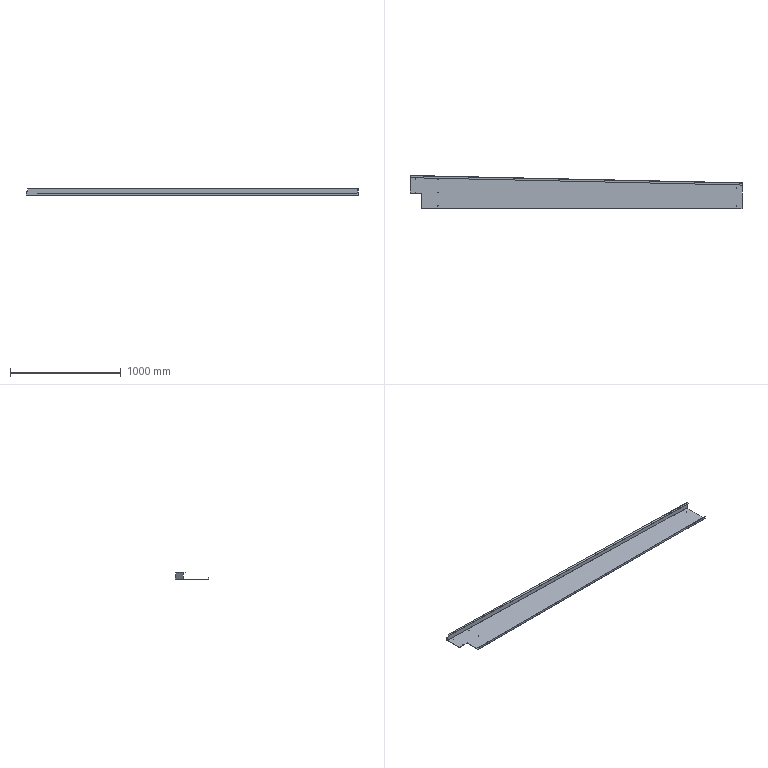Part | STEP file | TS-S53 | 1 solid | 49 faces | box 2995 x 298.377 x 60 mm | volume 2109135 mm3 | plane 28 | cylinder 20 | spline 1 | commonest cylinder face diameters 5.4 x14 0.4 x3 4.4 x3